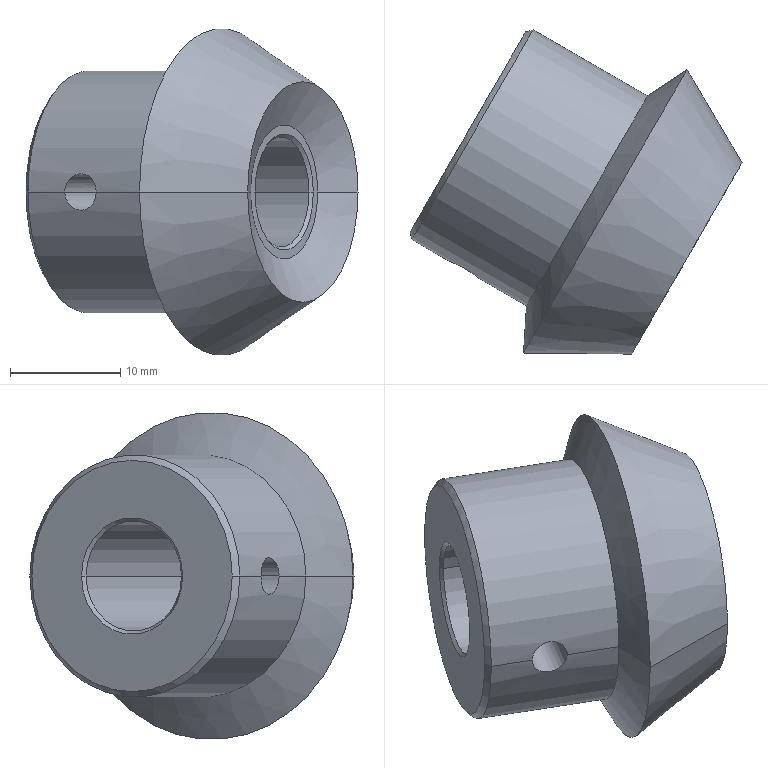Part | SolidWorks | features BaseBody 1 | 1 solid | 20 faces | box 30.143 x 29.432 x 29.68 mm | volume 7842 mm3 | cone 12 | cylinder 6 | plane 2 | commonest cylinder face diameters 3.3 x2 10 x2 22 x2
STEP:
#1=CARTESIAN_POINT('',(260.037,1759.86,-1178.57));
#2=VERTEX_POINT('',#1);
#3=CARTESIAN_POINT('',(249.037,1740.808,-1178.57));
#4=VERTEX_POINT('',#3);
#5=CARTESIAN_POINT('',(254.537,1750.334,-1178.57));
#6=DIRECTION('',(0.866,-0.5,0.));
#7=DIRECTION('',(0.5,0.866,0.));
#8=AXIS2_PLACEMENT_3D('',#5,#6,#7);
#9=CIRCLE('',#8,11.);
#10=EDGE_CURVE('',#2,#4,#9,.T.);
#11=ORIENTED_EDGE('',*,*,#10,.T.);
#12=CARTESIAN_POINT('',(252.371,1738.883,-1178.57));
#13=VERTEX_POINT('',#12);
#14=CARTESIAN_POINT('',(283.886,1720.688,-1178.57));
#15=DIRECTION('',(0.866,-0.5,0.));
#16=VECTOR('',#15,1000.);
#17=LINE('',#14,#16);
#18=EDGE_CURVE('',#4,#13,#17,.T.);
#19=ORIENTED_EDGE('',*,*,#18,.T.);
#20=CARTESIAN_POINT('',(255.229,1737.233,-1178.57));
#21=VERTEX_POINT('',#20);
#22=CARTESIAN_POINT('',(252.371,1738.883,-1178.57));
#23=CARTESIAN_POINT('',(252.371,1738.883,-1178.462));
#24=CARTESIAN_POINT('',(252.382,1738.879,-1178.353));
#25=CARTESIAN_POINT('',(252.421,1738.863,-1178.141));
#26=CARTESIAN_POINT('',(252.451,1738.851,-1178.038));
#27=CARTESIAN_POINT('',(252.528,1738.82,-1177.838));
#28=CARTESIAN_POINT('',(252.576,1738.8,-1177.742));
#29=CARTESIAN_POINT('',(252.687,1738.753,-1177.563));
#30=CARTESIAN_POINT('',(252.75,1738.726,-1177.48));
#31=CARTESIAN_POINT('',(252.892,1738.663,-1177.326));
#32=CARTESIAN_POINT('',(252.968,1738.629,-1177.258));
#33=CARTESIAN_POINT('',(253.13,1738.553,-1177.139));
#34=CARTESIAN_POINT('',(253.217,1738.51,-1177.087));
#35=CARTESIAN_POINT('',(253.485,1738.376,-1176.963));
#36=CARTESIAN_POINT('',(253.675,1738.274,-1176.92));
#37=CARTESIAN_POINT('',(253.958,1738.11,-1176.92));
#38=CARTESIAN_POINT('',(254.05,1738.055,-1176.931));
#39=CARTESIAN_POINT('',(254.23,1737.944,-1176.973));
#40=CARTESIAN_POINT('',(254.318,1737.888,-1177.005));
#41=CARTESIAN_POINT('',(254.485,1737.778,-1177.088));
#42=CARTESIAN_POINT('',(254.564,1737.725,-1177.139));
#43=CARTESIAN_POINT('',(254.712,1737.622,-1177.259));
#44=CARTESIAN_POINT('',(254.781,1737.573,-1177.328));
#45=CARTESIAN_POINT('',(254.966,1737.438,-1177.556));
#46=CARTESIAN_POINT('',(255.064,1737.362,-1177.74));
#47=CARTESIAN_POINT('',(255.195,1737.26,-1178.137));
#48=CARTESIAN_POINT('',(255.229,1737.233,-1178.354));
#49=CARTESIAN_POINT('',(255.229,1737.233,-1178.57));
#50=B_SPLINE_CURVE_WITH_KNOTS('',3,(#22,#23,#24,#25,#26,#27,#28,#29,#30,#31,#32,#33,#34,#35,#36,#37,#38,#39,#40,#41,#42,#43,#44,#45,#46,#47,#48,#49),.UNSPECIFIED.,.F.,.F.,(4,2,2,2,2,2,2,2,2,2,2,2,2,4),(0.007748,0.008071,0.008394,0.008717,0.009039,0.009362,0.009685,0.01033,0.01065,0.01098,0.0113,0.01162,0.01227,0.01291),.UNSPECIFIED.);
#51=EDGE_CURVE('',#13,#21,#50,.T.);
#52=ORIENTED_EDGE('',*,*,#51,.T.);
#53=CARTESIAN_POINT('',(259.429,1734.808,-1178.57));
#54=VERTEX_POINT('',#53);
#55=CARTESIAN_POINT('',(283.886,1720.688,-1178.57));
#56=DIRECTION('',(0.866,-0.5,0.));
#57=VECTOR('',#56,1000.);
#58=LINE('',#55,#57);
#59=EDGE_CURVE('',#21,#54,#58,.T.);
#60=ORIENTED_EDGE('',*,*,#59,.T.);
#61=CARTESIAN_POINT('',(270.429,1753.86,-1178.57));
#62=VERTEX_POINT('',#61);
#63=CARTESIAN_POINT('',(264.929,1744.334,-1178.57));
#64=DIRECTION('',(-0.866,0.5,0.));
#65=DIRECTION('',(0.5,0.866,0.));
#66=AXIS2_PLACEMENT_3D('',#63,#64,#65);
#67=CIRCLE('',#66,11.);
#68=EDGE_CURVE('',#54,#62,#67,.T.);
#69=ORIENTED_EDGE('',*,*,#68,.T.);
#70=CARTESIAN_POINT('',(294.886,1739.74,-1178.57));
#71=DIRECTION('',(0.866,-0.5,0.));
#72=VECTOR('',#71,1000.);
#73=LINE('',#70,#72);
#74=EDGE_CURVE('',#2,#62,#73,.T.);
#75=ORIENTED_EDGE('',*,*,#74,.F.);
#76=EDGE_LOOP('',(#11,#19,#52,#60,#69,#75));
#77=FACE_OUTER_BOUND('',#76,.T.);
#78=CARTESIAN_POINT('',(289.386,1730.214,-1178.57));
#79=DIRECTION('',(0.866,-0.5,0.));
#80=DIRECTION('',(0.5,0.866,0.));
#81=AXIS2_PLACEMENT_3D('',#78,#79,#80);
#82=CYLINDRICAL_SURFACE('',#81,11.);
#83=ADVANCED_FACE('',(#77),#82,.T.);
#84=CARTESIAN_POINT('',(259.354,1759.677,-1178.57));
#85=VERTEX_POINT('',#84);
#86=CARTESIAN_POINT('',(248.854,1741.491,-1178.57));
#87=VERTEX_POINT('',#86);
#88=CARTESIAN_POINT('',(254.104,1750.584,-1178.57));
#89=DIRECTION('',(0.866,-0.5,0.));
#90=DIRECTION('',(0.5,0.866,0.));
#91=AXIS2_PLACEMENT_3D('',#88,#89,#90);
#92=CIRCLE('',#91,10.5);
#93=EDGE_CURVE('',#85,#87,#92,.T.);
#94=ORIENTED_EDGE('',*,*,#93,.T.);
#95=CARTESIAN_POINT('',(249.037,1740.808,-1178.57));
#96=DIRECTION('',(0.2588,-0.9659,0.));
#97=VECTOR('',#96,1000.);
#98=LINE('',#95,#97);
#99=EDGE_CURVE('',#87,#4,#98,.T.);
#100=ORIENTED_EDGE('',*,*,#99,.T.);
#101=ORIENTED_EDGE('',*,*,#10,.F.);
#102=CARTESIAN_POINT('',(260.037,1759.86,-1178.57));
#103=DIRECTION('',(0.9659,0.2588,0.));
#104=VECTOR('',#103,1000.);
#105=LINE('',#102,#104);
#106=EDGE_CURVE('',#85,#2,#105,.T.);
#107=ORIENTED_EDGE('',*,*,#106,.F.);
#108=EDGE_LOOP('',(#94,#100,#101,#107));
#109=FACE_OUTER_BOUND('',#108,.T.);
#110=CARTESIAN_POINT('',(254.537,1750.334,-1178.57));
#111=DIRECTION('',(0.866,-0.5,0.));
#112=DIRECTION('',(0.5,0.866,0.));
#113=AXIS2_PLACEMENT_3D('',#110,#111,#112);
#114=CONICAL_SURFACE('',#113,11.,0.7854);
#115=ADVANCED_FACE('',(#109),#114,.T.);
#116=ORIENTED_EDGE('',*,*,#68,.F.);
#117=CARTESIAN_POINT('',(259.164,1730.527,-1178.57));
#118=VERTEX_POINT('',#117);
#119=CARTESIAN_POINT('',(259.164,1730.527,-1178.57));
#120=DIRECTION('',(-0.062,-0.9981,0.));
#121=VECTOR('',#120,1000.);
#122=LINE('',#119,#121);
#123=EDGE_CURVE('',#54,#118,#122,.T.);
#124=ORIENTED_EDGE('',*,*,#123,.T.);
#125=CARTESIAN_POINT('',(274.004,1756.231,-1178.57));
#126=VERTEX_POINT('',#125);
#127=CARTESIAN_POINT('',(266.584,1743.379,-1178.57));
#128=DIRECTION('',(-0.866,0.5,0.));
#129=DIRECTION('',(0.,0.,1.));
#130=AXIS2_PLACEMENT_3D('',#127,#128,#129);
#131=CIRCLE('',#130,14.84);
#132=EDGE_CURVE('',#118,#126,#131,.T.);
#133=ORIENTED_EDGE('',*,*,#132,.T.);
#134=CARTESIAN_POINT('',(274.004,1756.231,-1178.57));
#135=DIRECTION('',(0.8334,0.5527,0.));
#136=VECTOR('',#135,1000.);
#137=LINE('',#134,#136);
#138=EDGE_CURVE('',#62,#126,#137,.T.);
#139=ORIENTED_EDGE('',*,*,#138,.F.);
#140=EDGE_LOOP('',(#116,#124,#133,#139));
#141=FACE_OUTER_BOUND('',#140,.T.);
#142=CARTESIAN_POINT('',(266.584,1743.379,-1178.57));
#143=DIRECTION('',(0.866,-0.5,0.));
#144=DIRECTION('',(0.5,0.866,0.));
#145=AXIS2_PLACEMENT_3D('',#142,#143,#144);
#146=CONICAL_SURFACE('',#145,14.84,1.109);
#147=ADVANCED_FACE('',(#141),#146,.T.);
#148=CARTESIAN_POINT('',(255.371,1744.079,-1178.57));
#149=VERTEX_POINT('',#148);
#150=CARTESIAN_POINT('',(258.229,1742.429,-1178.57));
#151=VERTEX_POINT('',#150);
#152=CARTESIAN_POINT('',(255.371,1744.079,-1178.57));
#153=CARTESIAN_POINT('',(255.371,1744.079,-1178.678));
#154=CARTESIAN_POINT('',(255.383,1744.077,-1178.789));
#155=CARTESIAN_POINT('',(255.427,1744.067,-1179.001));
#156=CARTESIAN_POINT('',(255.459,1744.06,-1179.104));
#157=CARTESIAN_POINT('',(255.587,1744.031,-1179.405));
#158=CARTESIAN_POINT('',(255.71,1744.001,-1179.586));
#159=CARTESIAN_POINT('',(255.935,1743.934,-1179.814));
#160=CARTESIAN_POINT('',(256.015,1743.909,-1179.881));
#161=CARTESIAN_POINT('',(256.187,1743.849,-1180.001));
#162=CARTESIAN_POINT('',(256.278,1743.815,-1180.052));
#163=CARTESIAN_POINT('',(256.556,1743.7,-1180.176));
#164=CARTESIAN_POINT('',(256.752,1743.605,-1180.22));
#165=CARTESIAN_POINT('',(257.037,1743.441,-1180.22));
#166=CARTESIAN_POINT('',(257.128,1743.383,-1180.209));
#167=CARTESIAN_POINT('',(257.305,1743.265,-1180.166));
#168=CARTESIAN_POINT('',(257.39,1743.203,-1180.134));
#169=CARTESIAN_POINT('',(257.549,1743.08,-1180.051));
#170=CARTESIAN_POINT('',(257.623,1743.019,-1180.));
#171=CARTESIAN_POINT('',(257.761,1742.901,-1179.88));
#172=CARTESIAN_POINT('',(257.824,1742.843,-1179.811));
#173=CARTESIAN_POINT('',(257.993,1742.682,-1179.584));
#174=CARTESIAN_POINT('',(258.081,1742.59,-1179.402));
#175=CARTESIAN_POINT('',(258.169,1742.495,-1179.104));
#176=CARTESIAN_POINT('',(258.192,1742.47,-1178.999));
#177=CARTESIAN_POINT('',(258.222,1742.437,-1178.786));
#178=CARTESIAN_POINT('',(258.229,1742.429,-1178.678));
#179=CARTESIAN_POINT('',(258.229,1742.429,-1178.57));
#180=B_SPLINE_CURVE_WITH_KNOTS('',3,(#152,#153,#154,#155,#156,#157,#158,#159,#160,#161,#162,#163,#164,#165,#166,#167,#168,#169,#170,#171,#172,#173,#174,#175,#176,#177,#178,#179),.UNSPECIFIED.,.F.,.F.,(4,2,2,2,2,2,2,2,2,2,2,2,2,4),(0.007791,0.008116,0.008441,0.00909,0.009414,0.009739,0.01039,0.01071,0.01104,0.01136,0.01169,0.01234,0.01266,0.01298),.UNSPECIFIED.);
#181=EDGE_CURVE('',#149,#151,#180,.T.);
#182=ORIENTED_EDGE('',*,*,#181,.F.);
#183=CARTESIAN_POINT('',(252.371,1738.883,-1178.57));
#184=DIRECTION('',(-0.5,-0.866,0.));
#185=VECTOR('',#184,1000.);
#186=LINE('',#183,#185);
#187=EDGE_CURVE('',#149,#13,#186,.T.);
#188=ORIENTED_EDGE('',*,*,#187,.T.);
#189=CARTESIAN_POINT('',(255.229,1737.233,-1178.57));
#190=CARTESIAN_POINT('',(255.229,1737.233,-1178.678));
#191=CARTESIAN_POINT('',(255.221,1737.24,-1178.787));
#192=CARTESIAN_POINT('',(255.187,1737.266,-1178.999));
#193=CARTESIAN_POINT('',(255.162,1737.286,-1179.102));
#194=CARTESIAN_POINT('',(255.096,1737.337,-1179.302));
#195=CARTESIAN_POINT('',(255.055,1737.369,-1179.398));
#196=CARTESIAN_POINT('',(254.959,1737.441,-1179.577));
#197=CARTESIAN_POINT('',(254.904,1737.483,-1179.66));
#198=CARTESIAN_POINT('',(254.779,1737.574,-1179.814));
#199=CARTESIAN_POINT('',(254.711,1737.622,-1179.882));
#200=CARTESIAN_POINT('',(254.564,1737.725,-1180.001));
#201=CARTESIAN_POINT('',(254.484,1737.779,-1180.053));
#202=CARTESIAN_POINT('',(254.233,1737.944,-1180.177));
#203=CARTESIAN_POINT('',(254.051,1738.057,-1180.22));
#204=CARTESIAN_POINT('',(253.767,1738.221,-1180.22));
#205=CARTESIAN_POINT('',(253.673,1738.273,-1180.209));
#206=CARTESIAN_POINT('',(253.487,1738.373,-1180.167));
#207=CARTESIAN_POINT('',(253.394,1738.421,-1180.135));
#208=CARTESIAN_POINT('',(253.215,1738.511,-1180.052));
#209=CARTESIAN_POINT('',(253.13,1738.553,-1180.001));
#210=CARTESIAN_POINT('',(252.967,1738.629,-1179.881));
#211=CARTESIAN_POINT('',(252.89,1738.664,-1179.812));
#212=CARTESIAN_POINT('',(252.681,1738.757,-1179.584));
#213=CARTESIAN_POINT('',(252.566,1738.804,-1179.4));
#214=CARTESIAN_POINT('',(252.412,1738.867,-1179.003));
#215=CARTESIAN_POINT('',(252.371,1738.883,-1178.786));
#216=CARTESIAN_POINT('',(252.371,1738.883,-1178.57));
#217=B_SPLINE_CURVE_WITH_KNOTS('',3,(#189,#190,#191,#192,#193,#194,#195,#196,#197,#198,#199,#200,#201,#202,#203,#204,#205,#206,#207,#208,#209,#210,#211,#212,#213,#214,#215,#216),.UNSPECIFIED.,.F.,.F.,(4,2,2,2,2,2,2,2,2,2,2,2,2,4),(0.002584,0.002906,0.003229,0.003552,0.003875,0.004198,0.00452,0.005166,0.005489,0.005812,0.006134,0.006457,0.007103,0.007748),.UNSPECIFIED.);
#218=EDGE_CURVE('',#21,#13,#217,.T.);
#219=ORIENTED_EDGE('',*,*,#218,.F.);
#220=CARTESIAN_POINT('',(255.229,1737.233,-1178.57));
#221=DIRECTION('',(-0.5,-0.866,0.));
#222=VECTOR('',#221,1000.);
#223=LINE('',#220,#222);
#224=EDGE_CURVE('',#151,#21,#223,.T.);
#225=ORIENTED_EDGE('',*,*,#224,.F.);
#226=EDGE_LOOP('',(#182,#188,#219,#225));
#227=FACE_OUTER_BOUND('',#226,.T.);
#228=CARTESIAN_POINT('',(253.8,1738.058,-1178.57));
#229=DIRECTION('',(-0.5,-0.866,0.));
#230=DIRECTION('',(0.866,-0.5,0.));
#231=AXIS2_PLACEMENT_3D('',#228,#229,#230);
#232=CYLINDRICAL_SURFACE('',#231,1.65);
#233=ADVANCED_FACE('',(#227),#232,.F.);
#234=CARTESIAN_POINT('',(268.979,1730.428,-1178.57));
#235=VERTEX_POINT('',#234);
#236=CARTESIAN_POINT('',(278.997,1747.78,-1178.57));
#237=VERTEX_POINT('',#236);
#238=CARTESIAN_POINT('',(273.988,1739.104,-1178.57));
#239=DIRECTION('',(-0.866,0.5,0.));
#240=DIRECTION('',(0.,0.,-1.));
#241=AXIS2_PLACEMENT_3D('',#238,#239,#240);
#242=CIRCLE('',#241,10.018);
#243=EDGE_CURVE('',#235,#237,#242,.T.);
#244=ORIENTED_EDGE('',*,*,#243,.T.);
#245=CARTESIAN_POINT('',(274.004,1756.231,-1178.57));
#246=DIRECTION('',(-0.5087,0.8609,0.));
#247=VECTOR('',#246,1000.);
#248=LINE('',#245,#247);
#249=EDGE_CURVE('',#237,#126,#248,.T.);
#250=ORIENTED_EDGE('',*,*,#249,.T.);
#251=ORIENTED_EDGE('',*,*,#132,.F.);
#252=CARTESIAN_POINT('',(259.164,1730.527,-1178.57));
#253=DIRECTION('',(-0.9999,0.01012,0.));
#254=VECTOR('',#253,1000.);
#255=LINE('',#252,#254);
#256=EDGE_CURVE('',#235,#118,#255,.T.);
#257=ORIENTED_EDGE('',*,*,#256,.F.);
#258=EDGE_LOOP('',(#244,#250,#251,#257));
#259=FACE_OUTER_BOUND('',#258,.T.);
#260=CARTESIAN_POINT('',(266.584,1743.379,-1178.57));
#261=DIRECTION('',(-0.866,0.5,0.));
#262=DIRECTION('',(-0.5,-0.866,0.));
#263=AXIS2_PLACEMENT_3D('',#260,#261,#262);
#264=CONICAL_SURFACE('',#263,14.84,0.5135);
#265=ADVANCED_FACE('',(#259),#264,.T.);
#266=CARTESIAN_POINT('',(256.864,1754.764,-1178.57));
#267=VERTEX_POINT('',#266);
#268=CARTESIAN_POINT('',(251.864,1746.104,-1178.57));
#269=VERTEX_POINT('',#268);
#270=CARTESIAN_POINT('',(254.364,1750.434,-1178.57));
#271=DIRECTION('',(-0.866,0.5,0.));
#272=DIRECTION('',(0.,0.,-1.));
#273=AXIS2_PLACEMENT_3D('',#270,#271,#272);
#274=CIRCLE('',#273,5.);
#275=EDGE_CURVE('',#267,#269,#274,.T.);
#276=ORIENTED_EDGE('',*,*,#275,.F.);
#277=CARTESIAN_POINT('',(256.754,1755.174,-1178.57));
#278=VERTEX_POINT('',#277);
#279=CARTESIAN_POINT('',(256.754,1755.174,-1178.57));
#280=DIRECTION('',(-0.2588,0.9659,0.));
#281=VECTOR('',#280,1000.);
#282=LINE('',#279,#281);
#283=EDGE_CURVE('',#267,#278,#282,.T.);
#284=ORIENTED_EDGE('',*,*,#283,.T.);
#285=CARTESIAN_POINT('',(251.454,1745.994,-1178.57));
#286=VERTEX_POINT('',#285);
#287=CARTESIAN_POINT('',(254.104,1750.584,-1178.57));
#288=DIRECTION('',(-0.866,0.5,0.));
#289=DIRECTION('',(-0.5,-0.866,0.));
#290=AXIS2_PLACEMENT_3D('',#287,#288,#289);
#291=CIRCLE('',#290,5.3);
#292=EDGE_CURVE('',#278,#286,#291,.T.);
#293=ORIENTED_EDGE('',*,*,#292,.T.);
#294=CARTESIAN_POINT('',(251.454,1745.994,-1178.57));
#295=DIRECTION('',(-0.9659,-0.2588,0.));
#296=VECTOR('',#295,1000.);
#297=LINE('',#294,#296);
#298=EDGE_CURVE('',#269,#286,#297,.T.);
#299=ORIENTED_EDGE('',*,*,#298,.F.);
#300=EDGE_LOOP('',(#276,#284,#293,#299));
#301=FACE_OUTER_BOUND('',#300,.T.);
#302=CARTESIAN_POINT('',(254.104,1750.584,-1178.57));
#303=DIRECTION('',(-0.866,0.5,0.));
#304=DIRECTION('',(-0.5,-0.866,0.));
#305=AXIS2_PLACEMENT_3D('',#302,#303,#304);
#306=CONICAL_SURFACE('',#305,5.3,0.7854);
#307=ADVANCED_FACE('',(#301),#306,.F.);
#308=ORIENTED_EDGE('',*,*,#275,.T.);
#309=CARTESIAN_POINT('',(286.886,1725.884,-1178.57));
#310=DIRECTION('',(0.866,-0.5,0.));
#311=VECTOR('',#310,1000.);
#312=LINE('',#309,#311);
#313=EDGE_CURVE('',#269,#149,#312,.T.);
#314=ORIENTED_EDGE('',*,*,#313,.T.);
#315=ORIENTED_EDGE('',*,*,#181,.T.);
#316=CARTESIAN_POINT('',(269.531,1735.904,-1178.57));
#317=VERTEX_POINT('',#316);
#318=CARTESIAN_POINT('',(286.886,1725.884,-1178.57));
#319=DIRECTION('',(0.866,-0.5,0.));
#320=VECTOR('',#319,1000.);
#321=LINE('',#318,#320);
#322=EDGE_CURVE('',#151,#317,#321,.T.);
#323=ORIENTED_EDGE('',*,*,#322,.T.);
#324=CARTESIAN_POINT('',(274.531,1744.564,-1178.57));
#325=VERTEX_POINT('',#324);
#326=CARTESIAN_POINT('',(272.031,1740.234,-1178.57));
#327=DIRECTION('',(-0.866,0.5,0.));
#328=DIRECTION('',(0.5,0.866,0.));
#329=AXIS2_PLACEMENT_3D('',#326,#327,#328);
#330=CIRCLE('',#329,5.);
#331=EDGE_CURVE('',#325,#317,#330,.T.);
#332=ORIENTED_EDGE('',*,*,#331,.F.);
#333=CARTESIAN_POINT('',(291.886,1734.544,-1178.57));
#334=DIRECTION('',(0.866,-0.5,0.));
#335=VECTOR('',#334,1000.);
#336=LINE('',#333,#335);
#337=EDGE_CURVE('',#267,#325,#336,.T.);
#338=ORIENTED_EDGE('',*,*,#337,.F.);
#339=EDGE_LOOP('',(#308,#314,#315,#323,#332,#338));
#340=FACE_OUTER_BOUND('',#339,.T.);
#341=CARTESIAN_POINT('',(289.386,1730.214,-1178.57));
#342=DIRECTION('',(0.866,-0.5,0.));
#343=DIRECTION('',(0.5,0.866,0.));
#344=AXIS2_PLACEMENT_3D('',#341,#342,#343);
#345=CYLINDRICAL_SURFACE('',#344,5.);
#346=ADVANCED_FACE('',(#340),#345,.F.);
#347=CARTESIAN_POINT('',(269.241,1734.801,-1178.57));
#348=VERTEX_POINT('',#347);
#349=CARTESIAN_POINT('',(275.341,1745.367,-1178.57));
#350=VERTEX_POINT('',#349);
#351=CARTESIAN_POINT('',(272.291,1740.084,-1178.57));
#352=DIRECTION('',(0.866,-0.5,0.));
#353=DIRECTION('',(0.5,0.866,0.));
#354=AXIS2_PLACEMENT_3D('',#351,#352,#353);
#355=CIRCLE('',#354,6.1);
#356=EDGE_CURVE('',#348,#350,#355,.T.);
#357=ORIENTED_EDGE('',*,*,#356,.F.);
#358=CARTESIAN_POINT('',(268.979,1730.428,-1178.57));
#359=DIRECTION('',(-0.05975,-0.9982,0.));
#360=VECTOR('',#359,1000.);
#361=LINE('',#358,#360);
#362=EDGE_CURVE('',#348,#235,#361,.T.);
#363=ORIENTED_EDGE('',*,*,#362,.T.);
#364=CARTESIAN_POINT('',(273.988,1739.104,-1178.57));
#365=DIRECTION('',(-0.866,0.5,0.));
#366=DIRECTION('',(0.,0.,-1.));
#367=AXIS2_PLACEMENT_3D('',#364,#365,#366);
#368=CIRCLE('',#367,10.018);
#369=EDGE_CURVE('',#237,#235,#368,.T.);
#370=ORIENTED_EDGE('',*,*,#369,.F.);
#371=CARTESIAN_POINT('',(278.997,1747.78,-1178.57));
#372=DIRECTION('',(0.8346,0.5509,0.));
#373=VECTOR('',#372,1000.);
#374=LINE('',#371,#373);
#375=EDGE_CURVE('',#350,#237,#374,.T.);
#376=ORIENTED_EDGE('',*,*,#375,.F.);
#377=EDGE_LOOP('',(#357,#363,#370,#376));
#378=FACE_OUTER_BOUND('',#377,.T.);
#379=CARTESIAN_POINT('',(273.988,1739.104,-1178.57));
#380=DIRECTION('',(0.866,-0.5,0.));
#381=DIRECTION('',(0.5,0.866,0.));
#382=AXIS2_PLACEMENT_3D('',#379,#380,#381);
#383=CONICAL_SURFACE('',#382,10.018,1.107);
#384=ADVANCED_FACE('',(#378),#383,.F.);
#385=ORIENTED_EDGE('',*,*,#331,.T.);
#386=CARTESIAN_POINT('',(269.641,1735.494,-1178.57));
#387=VERTEX_POINT('',#386);
#388=CARTESIAN_POINT('',(269.641,1735.494,-1178.57));
#389=DIRECTION('',(0.2588,-0.9659,0.));
#390=VECTOR('',#389,1000.);
#391=LINE('',#388,#390);
#392=EDGE_CURVE('',#317,#387,#391,.T.);
#393=ORIENTED_EDGE('',*,*,#392,.T.);
#394=CARTESIAN_POINT('',(274.941,1744.674,-1178.57));
#395=VERTEX_POINT('',#394);
#396=CARTESIAN_POINT('',(272.291,1740.084,-1178.57));
#397=DIRECTION('',(-0.866,0.5,0.));
#398=DIRECTION('',(0.5,0.866,0.));
#399=AXIS2_PLACEMENT_3D('',#396,#397,#398);
#400=CIRCLE('',#399,5.3);
#401=EDGE_CURVE('',#395,#387,#400,.T.);
#402=ORIENTED_EDGE('',*,*,#401,.F.);
#403=CARTESIAN_POINT('',(274.941,1744.674,-1178.57));
#404=DIRECTION('',(0.9659,0.2588,0.));
#405=VECTOR('',#404,1000.);
#406=LINE('',#403,#405);
#407=EDGE_CURVE('',#325,#395,#406,.T.);
#408=ORIENTED_EDGE('',*,*,#407,.F.);
#409=EDGE_LOOP('',(#385,#393,#402,#408));
#410=FACE_OUTER_BOUND('',#409,.T.);
#411=CARTESIAN_POINT('',(272.291,1740.084,-1178.57));
#412=DIRECTION('',(0.866,-0.5,0.));
#413=DIRECTION('',(0.5,0.866,0.));
#414=AXIS2_PLACEMENT_3D('',#411,#412,#413);
#415=CONICAL_SURFACE('',#414,5.3,0.7854);
#416=ADVANCED_FACE('',(#410),#415,.F.);
#417=ORIENTED_EDGE('',*,*,#18,.F.);
#418=CARTESIAN_POINT('',(254.537,1750.334,-1178.57));
#419=DIRECTION('',(0.866,-0.5,0.));
#420=DIRECTION('',(0.5,0.866,0.));
#421=AXIS2_PLACEMENT_3D('',#418,#419,#420);
#422=CIRCLE('',#421,11.);
#423=EDGE_CURVE('',#4,#2,#422,.T.);
#424=ORIENTED_EDGE('',*,*,#423,.T.);
#425=ORIENTED_EDGE('',*,*,#74,.T.);
#426=CARTESIAN_POINT('',(264.929,1744.334,-1178.57));
#427=DIRECTION('',(-0.866,0.5,0.));
#428=DIRECTION('',(0.5,0.866,0.));
#429=AXIS2_PLACEMENT_3D('',#426,#427,#428);
#430=CIRCLE('',#429,11.);
#431=EDGE_CURVE('',#62,#54,#430,.T.);
#432=ORIENTED_EDGE('',*,*,#431,.T.);
#433=ORIENTED_EDGE('',*,*,#59,.F.);
#434=ORIENTED_EDGE('',*,*,#218,.T.);
#435=EDGE_LOOP('',(#417,#424,#425,#432,#433,#434));
#436=FACE_OUTER_BOUND('',#435,.T.);
#437=CARTESIAN_POINT('',(289.386,1730.214,-1178.57));
#438=DIRECTION('',(0.866,-0.5,0.));
#439=DIRECTION('',(0.5,0.866,0.));
#440=AXIS2_PLACEMENT_3D('',#437,#438,#439);
#441=CYLINDRICAL_SURFACE('',#440,11.);
#442=ADVANCED_FACE('',(#436),#441,.T.);
#443=ORIENTED_EDGE('',*,*,#99,.F.);
#444=CARTESIAN_POINT('',(254.104,1750.584,-1178.57));
#445=DIRECTION('',(0.866,-0.5,0.));
#446=DIRECTION('',(0.5,0.866,0.));
#447=AXIS2_PLACEMENT_3D('',#444,#445,#446);
#448=CIRCLE('',#447,10.5);
#449=EDGE_CURVE('',#87,#85,#448,.T.);
#450=ORIENTED_EDGE('',*,*,#449,.T.);
#451=ORIENTED_EDGE('',*,*,#106,.T.);
#452=ORIENTED_EDGE('',*,*,#423,.F.);
#453=EDGE_LOOP('',(#443,#450,#451,#452));
#454=FACE_OUTER_BOUND('',#453,.T.);
#455=CARTESIAN_POINT('',(254.537,1750.334,-1178.57));
#456=DIRECTION('',(0.866,-0.5,0.));
#457=DIRECTION('',(0.5,0.866,0.));
#458=AXIS2_PLACEMENT_3D('',#455,#456,#457);
#459=CONICAL_SURFACE('',#458,11.,0.7854);
#460=ADVANCED_FACE('',(#454),#459,.T.);
#461=ORIENTED_EDGE('',*,*,#123,.F.);
#462=ORIENTED_EDGE('',*,*,#431,.F.);
#463=ORIENTED_EDGE('',*,*,#138,.T.);
#464=CARTESIAN_POINT('',(266.584,1743.379,-1178.57));
#465=DIRECTION('',(-0.866,0.5,0.));
#466=DIRECTION('',(0.,0.,1.));
#467=AXIS2_PLACEMENT_3D('',#464,#465,#466);
#468=CIRCLE('',#467,14.84);
#469=EDGE_CURVE('',#126,#118,#468,.T.);
#470=ORIENTED_EDGE('',*,*,#469,.T.);
#471=EDGE_LOOP('',(#461,#462,#463,#470));
#472=FACE_OUTER_BOUND('',#471,.T.);
#473=CARTESIAN_POINT('',(266.584,1743.379,-1178.57));
#474=DIRECTION('',(0.866,-0.5,0.));
#475=DIRECTION('',(0.5,0.866,0.));
#476=AXIS2_PLACEMENT_3D('',#473,#474,#475);
#477=CONICAL_SURFACE('',#476,14.84,1.109);
#478=ADVANCED_FACE('',(#472),#477,.T.);
#479=CARTESIAN_POINT('',(254.104,1750.584,-1178.57));
#480=DIRECTION('',(-0.866,0.5,0.));
#481=DIRECTION('',(-0.5,-0.866,0.));
#482=AXIS2_PLACEMENT_3D('',#479,#480,#481);
#483=CIRCLE('',#482,5.3);
#484=EDGE_CURVE('',#286,#278,#483,.T.);
#485=ORIENTED_EDGE('',*,*,#484,.F.);
#486=ORIENTED_EDGE('',*,*,#292,.F.);
#487=EDGE_LOOP('',(#485,#486));
#488=FACE_BOUND('',#487,.T.);
#489=ORIENTED_EDGE('',*,*,#93,.F.);
#490=ORIENTED_EDGE('',*,*,#449,.F.);
#491=EDGE_LOOP('',(#489,#490));
#492=FACE_OUTER_BOUND('',#491,.T.);
#493=CARTESIAN_POINT('',(248.604,1741.058,-1178.57));
#494=DIRECTION('',(0.866,-0.5,0.));
#495=DIRECTION('',(0.5,0.866,0.));
#496=AXIS2_PLACEMENT_3D('',#493,#494,#495);
#497=PLANE('',#496);
#498=ADVANCED_FACE('',(#488,#492),#497,.F.);
#499=ORIENTED_EDGE('',*,*,#187,.F.);
#500=CARTESIAN_POINT('',(258.229,1742.429,-1178.57));
#501=CARTESIAN_POINT('',(258.229,1742.429,-1178.462));
#502=CARTESIAN_POINT('',(258.222,1742.438,-1178.351));
#503=CARTESIAN_POINT('',(258.192,1742.471,-1178.139));
#504=CARTESIAN_POINT('',(258.169,1742.495,-1178.036));
#505=CARTESIAN_POINT('',(258.08,1742.591,-1177.735));
#506=CARTESIAN_POINT('',(257.993,1742.683,-1177.554));
#507=CARTESIAN_POINT('',(257.822,1742.844,-1177.327));
#508=CARTESIAN_POINT('',(257.76,1742.901,-1177.259));
#509=CARTESIAN_POINT('',(257.623,1743.02,-1177.139));
#510=CARTESIAN_POINT('',(257.547,1743.082,-1177.088));
#511=CARTESIAN_POINT('',(257.309,1743.265,-1176.964));
#512=CARTESIAN_POINT('',(257.129,1743.388,-1176.92));
#513=CARTESIAN_POINT('',(256.844,1743.552,-1176.92));
#514=CARTESIAN_POINT('',(256.749,1743.603,-1176.931));
#515=CARTESIAN_POINT('',(256.558,1743.696,-1176.974));
#516=CARTESIAN_POINT('',(256.461,1743.739,-1177.006));
#517=CARTESIAN_POINT('',(256.276,1743.816,-1177.089));
#518=CARTESIAN_POINT('',(256.186,1743.849,-1177.14));
#519=CARTESIAN_POINT('',(256.014,1743.909,-1177.26));
#520=CARTESIAN_POINT('',(255.932,1743.935,-1177.329));
#521=CARTESIAN_POINT('',(255.709,1744.001,-1177.555));
#522=CARTESIAN_POINT('',(255.585,1744.031,-1177.738));
#523=CARTESIAN_POINT('',(255.459,1744.06,-1178.036));
#524=CARTESIAN_POINT('',(255.426,1744.067,-1178.141));
#525=CARTESIAN_POINT('',(255.382,1744.077,-1178.354));
#526=CARTESIAN_POINT('',(255.371,1744.079,-1178.462));
#527=CARTESIAN_POINT('',(255.371,1744.079,-1178.57));
#528=B_SPLINE_CURVE_WITH_KNOTS('',3,(#500,#501,#502,#503,#504,#505,#506,#507,#508,#509,#510,#511,#512,#513,#514,#515,#516,#517,#518,#519,#520,#521,#522,#523,#524,#525,#526,#527),.UNSPECIFIED.,.F.,.F.,(4,2,2,2,2,2,2,2,2,2,2,2,2,4),(0.002598,0.002923,0.003248,0.003897,0.004221,0.004546,0.005195,0.00552,0.005844,0.006169,0.006493,0.007142,0.007467,0.007791),.UNSPECIFIED.);
#529=EDGE_CURVE('',#151,#149,#528,.T.);
#530=ORIENTED_EDGE('',*,*,#529,.F.);
#531=ORIENTED_EDGE('',*,*,#224,.T.);
#532=ORIENTED_EDGE('',*,*,#51,.F.);
#533=EDGE_LOOP('',(#499,#530,#531,#532));
#534=FACE_OUTER_BOUND('',#533,.T.);
#535=CARTESIAN_POINT('',(253.8,1738.058,-1178.57));
#536=DIRECTION('',(-0.5,-0.866,0.));
#537=DIRECTION('',(0.866,-0.5,0.));
#538=AXIS2_PLACEMENT_3D('',#535,#536,#537);
#539=CYLINDRICAL_SURFACE('',#538,1.65);
#540=ADVANCED_FACE('',(#534),#539,.F.);
#541=ORIENTED_EDGE('',*,*,#249,.F.);
#542=ORIENTED_EDGE('',*,*,#369,.T.);
#543=ORIENTED_EDGE('',*,*,#256,.T.);
#544=ORIENTED_EDGE('',*,*,#469,.F.);
#545=EDGE_LOOP('',(#541,#542,#543,#544));
#546=FACE_OUTER_BOUND('',#545,.T.);
#547=CARTESIAN_POINT('',(266.584,1743.379,-1178.57));
#548=DIRECTION('',(-0.866,0.5,0.));
#549=DIRECTION('',(-0.5,-0.866,0.));
#550=AXIS2_PLACEMENT_3D('',#547,#548,#549);
#551=CONICAL_SURFACE('',#550,14.84,0.5135);
#552=ADVANCED_FACE('',(#546),#551,.T.);
#553=ORIENTED_EDGE('',*,*,#283,.F.);
#554=CARTESIAN_POINT('',(254.364,1750.434,-1178.57));
#555=DIRECTION('',(-0.866,0.5,0.));
#556=DIRECTION('',(0.,0.,-1.));
#557=AXIS2_PLACEMENT_3D('',#554,#555,#556);
#558=CIRCLE('',#557,5.);
#559=EDGE_CURVE('',#269,#267,#558,.T.);
#560=ORIENTED_EDGE('',*,*,#559,.F.);
#561=ORIENTED_EDGE('',*,*,#298,.T.);
#562=ORIENTED_EDGE('',*,*,#484,.T.);
#563=EDGE_LOOP('',(#553,#560,#561,#562));
#564=FACE_OUTER_BOUND('',#563,.T.);
#565=CARTESIAN_POINT('',(254.104,1750.584,-1178.57));
#566=DIRECTION('',(-0.866,0.5,0.));
#567=DIRECTION('',(-0.5,-0.866,0.));
#568=AXIS2_PLACEMENT_3D('',#565,#566,#567);
#569=CONICAL_SURFACE('',#568,5.3,0.7854);
#570=ADVANCED_FACE('',(#564),#569,.F.);
#571=ORIENTED_EDGE('',*,*,#313,.F.);
#572=ORIENTED_EDGE('',*,*,#559,.T.);
#573=ORIENTED_EDGE('',*,*,#337,.T.);
#574=CARTESIAN_POINT('',(272.031,1740.234,-1178.57));
#575=DIRECTION('',(-0.866,0.5,0.));
#576=DIRECTION('',(0.5,0.866,0.));
#577=AXIS2_PLACEMENT_3D('',#574,#575,#576);
#578=CIRCLE('',#577,5.);
#579=EDGE_CURVE('',#317,#325,#578,.T.);
#580=ORIENTED_EDGE('',*,*,#579,.F.);
#581=ORIENTED_EDGE('',*,*,#322,.F.);
#582=ORIENTED_EDGE('',*,*,#529,.T.);
#583=EDGE_LOOP('',(#571,#572,#573,#580,#581,#582));
#584=FACE_OUTER_BOUND('',#583,.T.);
#585=CARTESIAN_POINT('',(289.386,1730.214,-1178.57));
#586=DIRECTION('',(0.866,-0.5,0.));
#587=DIRECTION('',(0.5,0.866,0.));
#588=AXIS2_PLACEMENT_3D('',#585,#586,#587);
#589=CYLINDRICAL_SURFACE('',#588,5.);
#590=ADVANCED_FACE('',(#584),#589,.F.);
#591=ORIENTED_EDGE('',*,*,#362,.F.);
#592=CARTESIAN_POINT('',(272.291,1740.084,-1178.57));
#593=DIRECTION('',(0.866,-0.5,0.));
#594=DIRECTION('',(0.5,0.866,0.));
#595=AXIS2_PLACEMENT_3D('',#592,#593,#594);
#596=CIRCLE('',#595,6.1);
#597=EDGE_CURVE('',#350,#348,#596,.T.);
#598=ORIENTED_EDGE('',*,*,#597,.F.);
#599=ORIENTED_EDGE('',*,*,#375,.T.);
#600=ORIENTED_EDGE('',*,*,#243,.F.);
#601=EDGE_LOOP('',(#591,#598,#599,#600));
#602=FACE_OUTER_BOUND('',#601,.T.);
#603=CARTESIAN_POINT('',(273.988,1739.104,-1178.57));
#604=DIRECTION('',(0.866,-0.5,0.));
#605=DIRECTION('',(0.5,0.866,0.));
#606=AXIS2_PLACEMENT_3D('',#603,#604,#605);
#607=CONICAL_SURFACE('',#606,10.018,1.107);
#608=ADVANCED_FACE('',(#602),#607,.F.);
#609=ORIENTED_EDGE('',*,*,#392,.F.);
#610=ORIENTED_EDGE('',*,*,#579,.T.);
#611=ORIENTED_EDGE('',*,*,#407,.T.);
#612=CARTESIAN_POINT('',(272.291,1740.084,-1178.57));
#613=DIRECTION('',(-0.866,0.5,0.));
#614=DIRECTION('',(0.5,0.866,0.));
#615=AXIS2_PLACEMENT_3D('',#612,#613,#614);
#616=CIRCLE('',#615,5.3);
#617=EDGE_CURVE('',#387,#395,#616,.T.);
#618=ORIENTED_EDGE('',*,*,#617,.F.);
#619=EDGE_LOOP('',(#609,#610,#611,#618));
#620=FACE_OUTER_BOUND('',#619,.T.);
#621=CARTESIAN_POINT('',(272.291,1740.084,-1178.57));
#622=DIRECTION('',(0.866,-0.5,0.));
#623=DIRECTION('',(0.5,0.866,0.));
#624=AXIS2_PLACEMENT_3D('',#621,#622,#623);
#625=CONICAL_SURFACE('',#624,5.3,0.7854);
#626=ADVANCED_FACE('',(#620),#625,.F.);
#627=ORIENTED_EDGE('',*,*,#401,.T.);
#628=ORIENTED_EDGE('',*,*,#617,.T.);
#629=EDGE_LOOP('',(#627,#628));
#630=FACE_BOUND('',#629,.T.);
#631=ORIENTED_EDGE('',*,*,#597,.T.);
#632=ORIENTED_EDGE('',*,*,#356,.T.);
#633=EDGE_LOOP('',(#631,#632));
#634=FACE_OUTER_BOUND('',#633,.T.);
#635=CARTESIAN_POINT('',(269.791,1735.754,-1178.57));
#636=DIRECTION('',(-0.866,0.5,0.));
#637=DIRECTION('',(-0.5,-0.866,0.));
#638=AXIS2_PLACEMENT_3D('',#635,#636,#637);
#639=PLANE('',#638);
#640=ADVANCED_FACE('',(#630,#634),#639,.F.);
#641=CLOSED_SHELL('',(#83,#115,#147,#233,#265,#307,#346,#384,#416,#442,#460,#478,#498,#540,#552,#570,#590,#608,#626,#640));
#642=MANIFOLD_SOLID_BREP('',#641);
#643=CARTESIAN_POINT('',(0.,0.,0.));
#644=DIRECTION('',(0.,0.,1.));
#645=DIRECTION('',(1.,0.,0.));
#646=AXIS2_PLACEMENT_3D('',#643,#644,#645);
#647=(LENGTH_UNIT()NAMED_UNIT(*)SI_UNIT(.MILLI.,.METRE.));
#648=UNCERTAINTY_MEASURE_WITH_UNIT(LENGTH_MEASURE(0.00001),#647,'','');
#649=(NAMED_UNIT(*)PLANE_ANGLE_UNIT()SI_UNIT($,.RADIAN.));
#650=(NAMED_UNIT(*)SI_UNIT($,.STERADIAN.)SOLID_ANGLE_UNIT());
#651=(GEOMETRIC_REPRESENTATION_CONTEXT(3)GLOBAL_UNCERTAINTY_ASSIGNED_CONTEXT((#648))GLOBAL_UNIT_ASSIGNED_CONTEXT((#647,#649,#650))REPRESENTATION_CONTEXT('',''));
#652=ADVANCED_BREP_SHAPE_REPRESENTATION('',(#642,#646),#651);